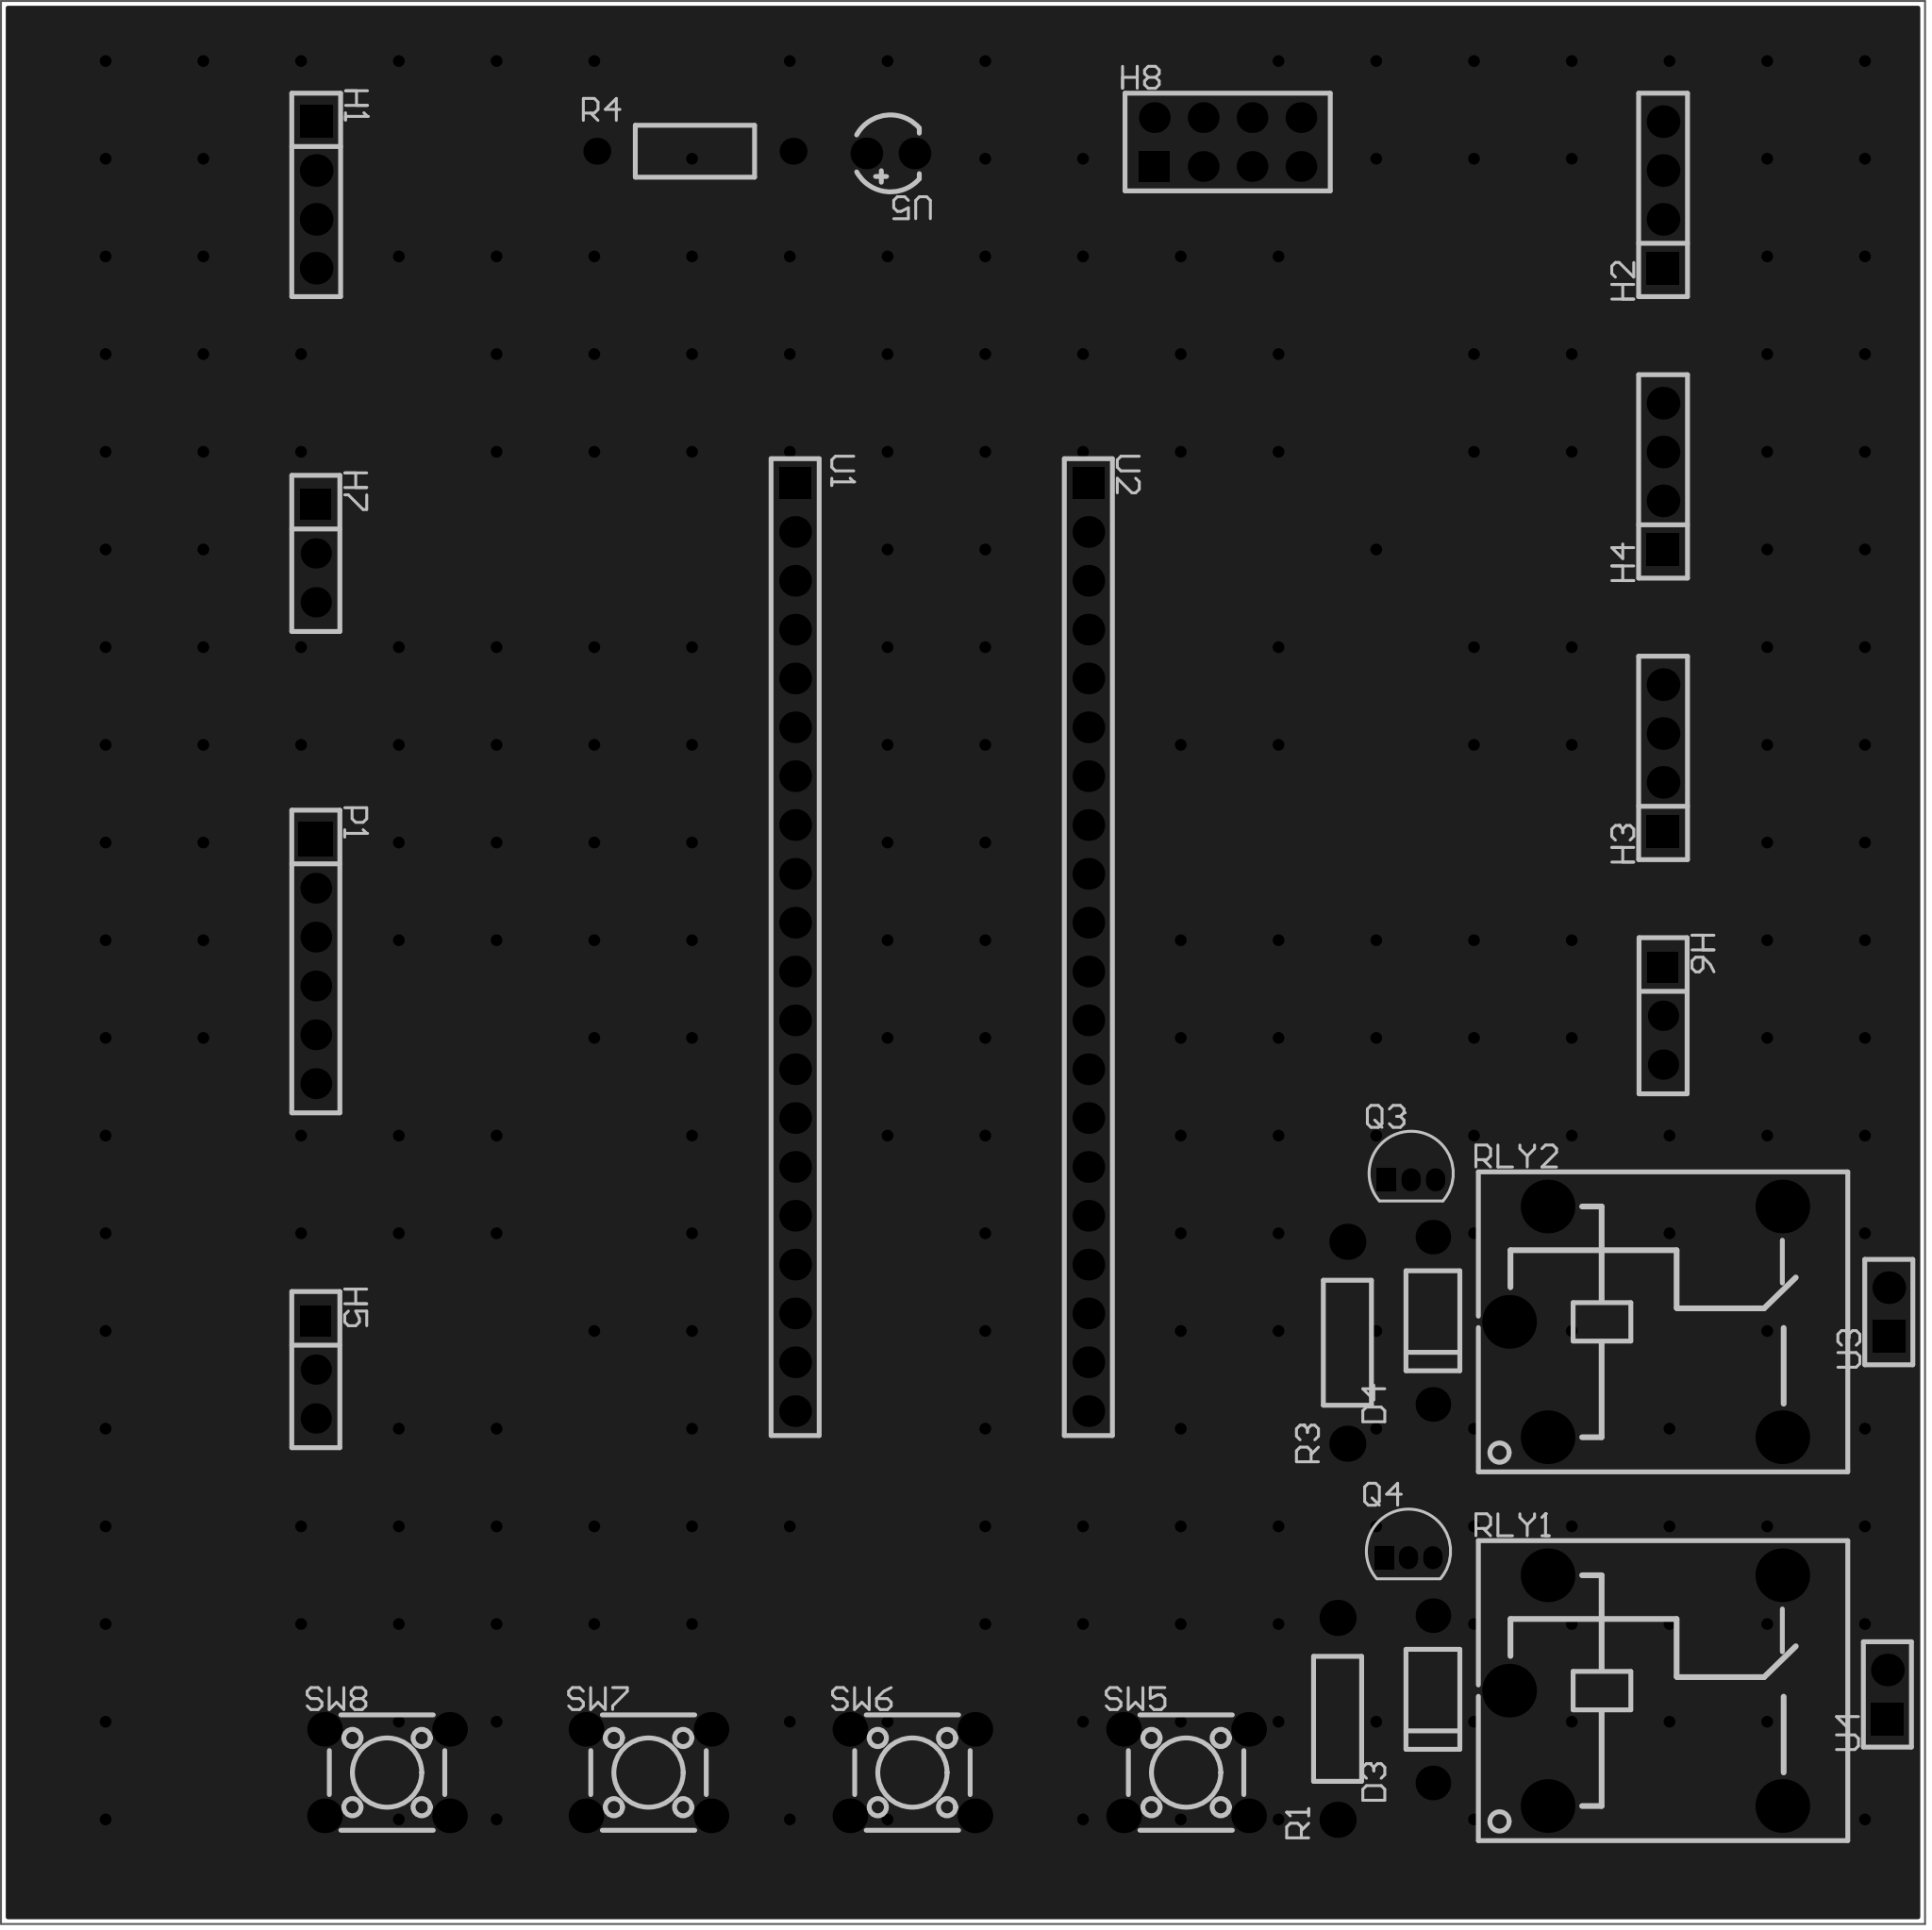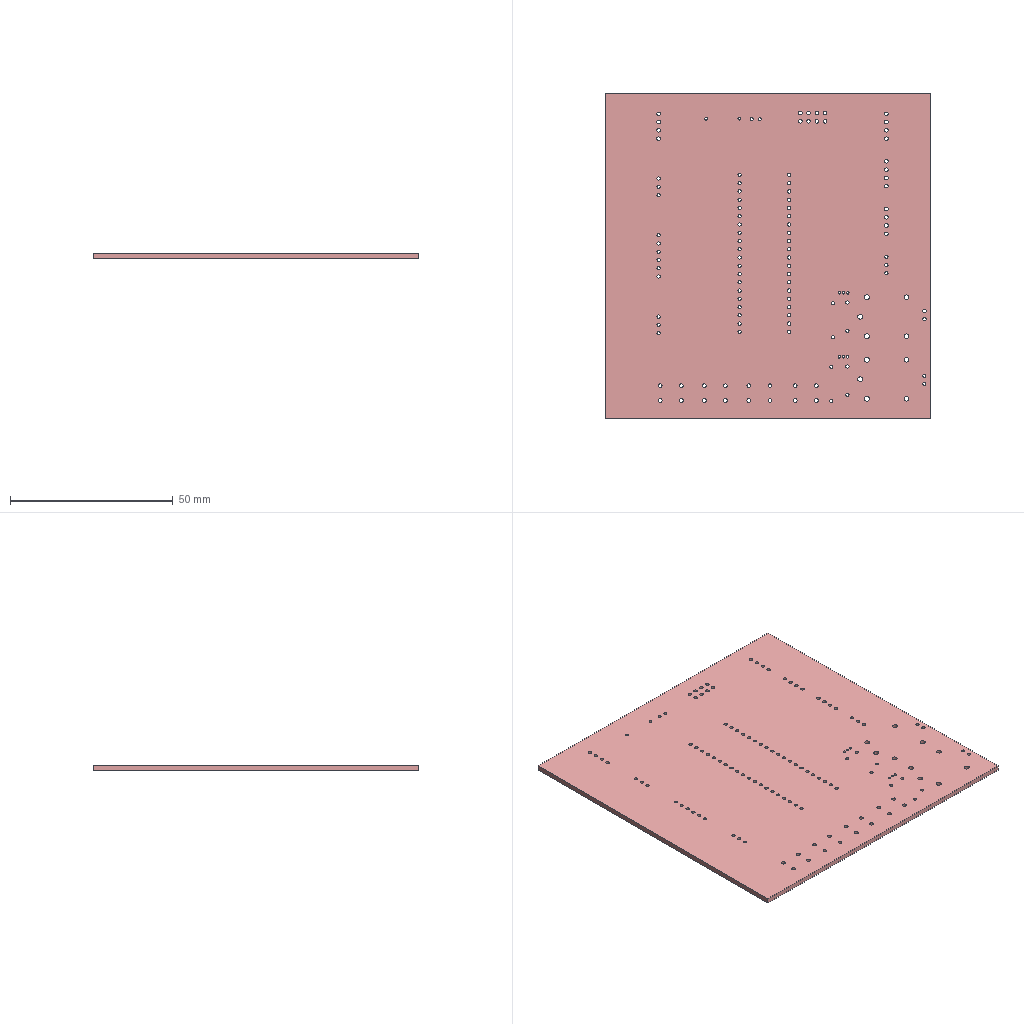Circuit board layout | Altium Designer | box 100 x 100 x 1.6 mm
Layer stack:
# Altium Designer layer stack of  (unit mm; dielectric type: 0 none, 1 core, 2 prepreg, 3 surface material)
index,name,kind,layer,copper_thickness_mm,dielectric_type,dielectric_thickness_mm,dielectric_material,dielectric_constant
0,Top Paste Mask Layer,other,,,,,,
1,Top Silkscreen Layer,other,,,,,,
2,Top Solder Mask Layer,dielectric,,,3,0.01,,3.3
3,Top Layer,copper,Top Layer,0.035,,,,
4,Dielectric1,dielectric,,,3,1.51,FR4,4.5
5,Bottom Layer,copper,Bottom Layer,0.035,,,,
6,Bottom Solder Mask Layer,dielectric,,,3,0.01,,3.3
7,Bottom Silkscreen Layer,other,,,,,,
8,Bottom Paste Mask Layer,other,,,,,,
# drill layer pairs: low layer,high layer
drill_pair,Top Layer,Bottom Layer
Part placement:
Designator,Comment,Layer,Footprint,Center-X(mm),Center-Y(mm),Rotation
H1,oled,TopLayer,HDR-TH_4P-P2.54-V-F,107.95,174.752,270
H2,mq2,TopLayer,HDR-TH_4P-P2.54-V-F,177.952,174.752,90
H3,mq7,TopLayer,HDR-TH_4P-P2.54-V-F,177.952,145.475,90
H4,mq135,TopLayer,HDR-TH_4P-P2.54-V-F,177.952,160.113,90
H5,Buzzer,TopLayer,HDR-TH_3P-P2.54-V-F,107.93,113.665,270
H6,Photoresistor,TopLayer,HDR-TH_3P-P2.54-V-F,177.952,132.066,270
H7,dht22,TopLayer,HDR-TH_3P-P2.54-V-F,107.93,156.11,270
P1,uln2003,TopLayer,HDR-TH_6P-P2.54-V-F,107.93,134.887,270
RLY1,SRD-05VDC-SL-C,TopLayer,RELAY-TH_SRD-XXVDC-XL-C,177.051,96.971,0
RLY2,SRD-05VDC-SL-C,TopLayer,RELAY-TH_SRD-XXVDC-XL-C,177.051,116.148,0
U1,KH-2.54FH-1X20P-H8.5,TopLayer,HDR-TH_20P-P2.54-V-F-2,132.842,135.636,270
U2,KH-2.54FH-1X20P-H8.5,TopLayer,HDR-TH_20P-P2.54-V-F-2,148.082,135.636,270
U3,Humidifier,TopLayer,HDR-TH_2P-P2.54-V-F,189.683,116.656,90
U4,Fan,TopLayer,HDR-TH_2P-P2.54-V-F,189.611,96.774,90
SW5,TC-00104-050E,TopLayer,SW-TH_4P-L6.0-W6.0-P4.50-LS6.5,153.162,92.71,0
SW6,TC-00104-050E,TopLayer,SW-TH_4P-L6.0-W6.0-P4.50-LS6.5,138.938,92.71,0
SW7,TC-00104-050E,TopLayer,SW-TH_4P-L6.0-W6.0-P4.50-LS6.5,125.222,92.71,0
SW8,TC-00104-050E,TopLayer,SW-TH_4P-L6.0-W6.0-P4.50-LS6.5,111.633,92.71,0
H8,esp8266,TopLayer,HDR-TH_8P-P2.54-V-F-R2-C4-S2.54,155.321,177.502,0
D3,1N4001,TopLayer,DO-41_BD2.4-L4.7-P8.70-D0.9-RD,165.989,96.52,90
D4,1N4001,TopLayer,DO-41_BD2.4-L4.7-P8.70-D0.9-RD,165.989,116.205,90
Q3,S8050,TopLayer,TO-92-3_L4.5-W3.5-P1.27-L,164.859,123.535,0
Q4,S8050,TopLayer,TO-92-3_L4.5-W3.5-P1.27-L,164.719,103.886,0
R1,1kΩ,TopLayer,RES-TH_BD2.5-L6.5-P10.50-D0.6,161.036,95.504,90
R3,1kΩ,TopLayer,RES-TH_BD2.5-L6.5-P10.50-D0.6,161.544,115.062,90
R4,10kΩ,TopLayer,RES-TH_BD2.7-L6.2-P10.20-D0.4,127.635,177.023,0
U5,204-10SDRD/S530-A3/F182-68,TopLayer,LED-TH_BD4.0-P2.50-RD,137.795,176.911,180
Pad and via stacks:
# Altium Designer via and pad stacks of  (unit mm). Each distinct definition once, with the count of objects using it.
# via: kind,start_layer,end_layer,hole_mm,diameter_mm,mode(0 simple;1 top-mid-bottom;2 full stack),diameter_per_layer,count,example_net
# pad: kind,layer,hole_mm,hole_type(0 round;1 square;2 slot),plating,top_size,top_shape(1 round;2 rect;3 octagon;9 rounded rect),mid_size,bottom_size,mode,footprint,size_per_layer,count,example
pad,Multi-Layer,1.1,0,plated,1.7x1.7,2,1.7x1.7,1.7x1.7,0,HDR-TH_4P-P2.54-V-F,,4,H1.1
pad,Multi-Layer,1.1,0,plated,1.7x1.7,1,1.7x1.7,1.7x1.7,0,HDR-TH_4P-P2.54-V-F,,12,H1.2
pad,Multi-Layer,1.02,0,plated,1.575x1.575,1,1.575x1.575,1.575x1.575,0,HDR-TH_3P-P2.54-V-F,,6,H5.3
pad,Multi-Layer,1.02,0,plated,1.575x1.575,2,1.575x1.575,1.575x1.575,0,HDR-TH_3P-P2.54-V-F,,3,H5.1
pad,Multi-Layer,1.02,0,plated,1.6x1.6,1,1.6x1.6,1.6x1.6,0,HDR-TH_6P-P2.54-V-F,,5,P1.6
pad,Multi-Layer,1.02,0,plated,1.8x1.8,2,1.8x1.8,1.8x1.8,0,HDR-TH_6P-P2.54-V-F,,1,P1.1
pad,Multi-Layer,1.524,0,plated,2.794x2.794,1,2.794x2.794,2.794x2.794,0,RELAY-TH_SRD-XXVDC-XL-C,,10,RLY1.2
pad,Multi-Layer,1.02,0,plated,1.65x1.65,2,1.65x1.65,1.65x1.65,0,HDR-TH_20P-P2.54-V-F-2,,2,U1.1
pad,Multi-Layer,1.02,0,plated,1.65x1.65,1,1.65x1.65,1.65x1.65,0,HDR-TH_20P-P2.54-V-F-2,,38,U1.2
pad,Multi-Layer,1,0,plated,1.7x1.7,2,1.7x1.7,1.7x1.7,0,HDR-TH_2P-P2.54-V-F,,2,U3.1
pad,Multi-Layer,1,0,plated,1.7x1.7,1,1.7x1.7,1.7x1.7,0,HDR-TH_2P-P2.54-V-F,,2,U3.2
pad,Multi-Layer,1.2,0,plated,1.8x1.8,1,1.8x1.8,1.8x1.8,0,SW-TH_4P-L6.0-W6.0-P4.50-LS6.5,,16,SW5.1
pad,Multi-Layer,1.1,0,plated,1.6x1.6,2,1.6x1.6,1.6x1.6,0,HDR-TH_8P-P2.54-V-F-R2-C4-S2.54,,1,H8.1
pad,Multi-Layer,1.1,0,plated,1.6x1.6,1,1.6x1.6,1.6x1.6,0,HDR-TH_8P-P2.54-V-F-R2-C4-S2.54,,7,H8.2
pad,Multi-Layer,1,0,plated,1.8x1.8,1,1.8x1.8,1.8x1.8,0,DO-41_BD2.4-L4.7-P8.70-D0.9-RD,,4,D3.1
pad,Multi-Layer,0.7,2,plated,1x1.2,2,1x1.2,1x1.2,0,TO-92-3_L4.5-W3.5-P1.27-L,,2,Q3.1
pad,Multi-Layer,0.7,2,plated,1x1.2,1,1x1.2,1x1.2,0,TO-92-3_L4.5-W3.5-P1.27-L,,4,Q3.2
pad,Multi-Layer,1,0,plated,1.88x1.88,1,1.88x1.88,1.88x1.88,0,RES-TH_BD2.5-L6.5-P10.50-D0.6,,4,R1.1
pad,Multi-Layer,0.8,0,plated,1.4x1.4,1,1.4x1.4,1.4x1.4,0,RES-TH_BD2.7-L6.2-P10.20-D0.4,,2,R4.1
pad,Multi-Layer,0.9,0,plated,1.651x1.651,1,1.651x1.651,1.651x1.651,0,LED-TH_BD4.0-P2.50-RD,,2,U5.2
via,Top Layer,Bottom Layer,0.3048,0.61,0,,246,GND
Copper pours:
name,layer,net,type(0 solid;1 hatched;2 none)
Top Layer-GND,Top Layer,GND,0
Bottom Layer-GND,Bottom Layer,GND,0